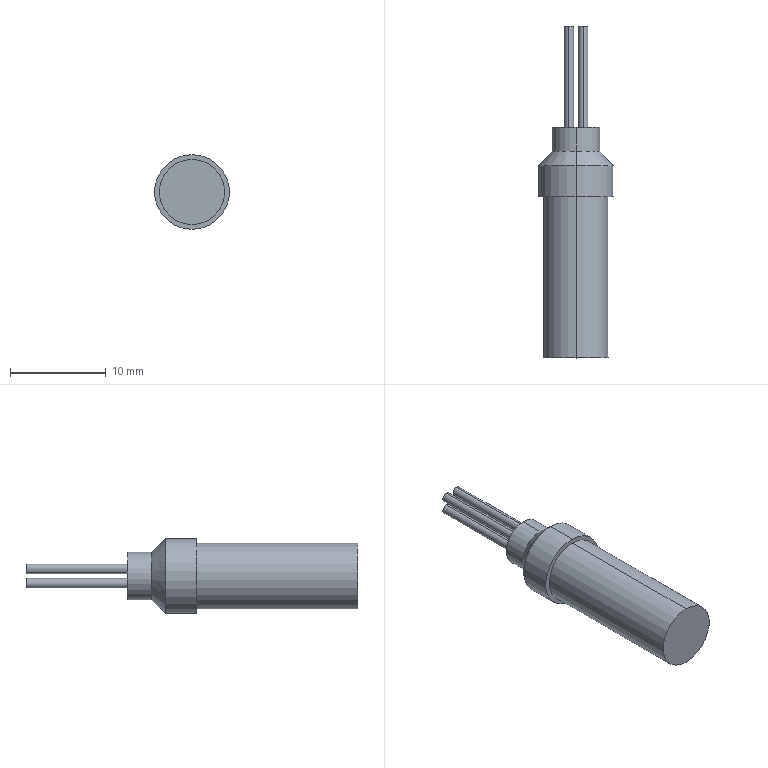Part | STEP file | Cable_Motor_Top_03_MSMF | 1 solid | 23 faces | box 7.8 x 34.633 x 7.8 mm | volume 896.959 mm3 | cylinder 14 | plane 7 | cone 2 | commonest cylinder face diameters 1 x8 5 x2 6.799 x2 7.8 x2
STEP:
#1=CARTESIAN_POINT('',(0.,0.,0.));
#2=DIRECTION('',(0.,0.,1.));
#3=DIRECTION('',(1.,0.,0.));
#4=AXIS2_PLACEMENT_3D('',#1,#2,#3);
#5=CARTESIAN_POINT('',(0.75,94.895,1.25));
#6=VERTEX_POINT('',#5);
#7=CARTESIAN_POINT('',(0.75,94.895,0.25));
#8=VERTEX_POINT('',#7);
#9=CARTESIAN_POINT('',(0.75,94.895,0.75));
#10=DIRECTION('',(0.,1.,0.));
#11=DIRECTION('',(0.,0.,1.));
#12=AXIS2_PLACEMENT_3D('',#9,#10,#11);
#13=CIRCLE('',#12,0.5);
#14=CARTESIAN_POINT('',(0.75,94.895,0.75));
#15=DIRECTION('',(0.,-1.,0.));
#16=DIRECTION('',(0.,0.,-1.));
#17=AXIS2_PLACEMENT_3D('',#14,#15,#16);
#18=CYLINDRICAL_SURFACE('',#17,0.5);
#19=CARTESIAN_POINT('',(3.142,0.));
#20=DIRECTION('',(-1.,0.));
#21=VECTOR('',#20,1.);
#22=LINE('',#19,#21);
#23=(GEOMETRIC_REPRESENTATION_CONTEXT(2)PARAMETRIC_REPRESENTATION_CONTEXT()REPRESENTATION_CONTEXT('',''));
#24=DEFINITIONAL_REPRESENTATION('',(#22),#23);
#25=PCURVE('',#18,#24);
#26=CARTESIAN_POINT('',(0.75,94.895,0.75));
#27=DIRECTION('',(0.,1.,0.));
#28=DIRECTION('',(0.,0.,1.));
#29=AXIS2_PLACEMENT_3D('',#26,#27,#28);
#30=PLANE('',#29);
#31=CARTESIAN_POINT('',(0.,0.));
#32=DIRECTION('',(1.,0.));
#33=AXIS2_PLACEMENT_2D('',#31,#32);
#34=CIRCLE('',#33,0.5);
#35=(GEOMETRIC_REPRESENTATION_CONTEXT(2)PARAMETRIC_REPRESENTATION_CONTEXT()REPRESENTATION_CONTEXT('',''));
#36=DEFINITIONAL_REPRESENTATION('',(#34),#35);
#37=PCURVE('',#30,#36);
#38=SURFACE_CURVE('',#13,(#25,#37),.PCURVE_S1.);
#39=EDGE_CURVE('',#6,#8,#38,.T.);
#40=ORIENTED_EDGE('',*,*,#39,.F.);
#41=CARTESIAN_POINT('',(0.75,84.322,1.25));
#42=VERTEX_POINT('',#41);
#43=CARTESIAN_POINT('',(0.75,94.895,1.25));
#44=DIRECTION('',(0.,-1.,0.));
#45=VECTOR('',#44,1.);
#46=LINE('',#43,#45);
#47=CARTESIAN_POINT('',(3.142,0.));
#48=DIRECTION('',(0.,1.));
#49=VECTOR('',#48,1.);
#50=LINE('',#47,#49);
#51=(GEOMETRIC_REPRESENTATION_CONTEXT(2)PARAMETRIC_REPRESENTATION_CONTEXT()REPRESENTATION_CONTEXT('',''));
#52=DEFINITIONAL_REPRESENTATION('',(#50),#51);
#53=PCURVE('',#18,#52);
#54=CARTESIAN_POINT('',(0.75,94.895,0.75));
#55=DIRECTION('',(0.,-1.,0.));
#56=DIRECTION('',(0.,0.,-1.));
#57=AXIS2_PLACEMENT_3D('',#54,#55,#56);
#58=CYLINDRICAL_SURFACE('',#57,0.5);
#59=CARTESIAN_POINT('',(3.142,0.));
#60=DIRECTION('',(0.,1.));
#61=VECTOR('',#60,1.);
#62=LINE('',#59,#61);
#63=(GEOMETRIC_REPRESENTATION_CONTEXT(2)PARAMETRIC_REPRESENTATION_CONTEXT()REPRESENTATION_CONTEXT('',''));
#64=DEFINITIONAL_REPRESENTATION('',(#62),#63);
#65=PCURVE('',#58,#64);
#66=SURFACE_CURVE('',#46,(#53,#65),.PCURVE_S1.);
#67=EDGE_CURVE('',#6,#42,#66,.T.);
#68=ORIENTED_EDGE('',*,*,#67,.T.);
#69=CARTESIAN_POINT('',(0.75,84.322,0.25));
#70=VERTEX_POINT('',#69);
#71=CARTESIAN_POINT('',(0.75,84.322,0.75));
#72=DIRECTION('',(0.,1.,0.));
#73=DIRECTION('',(0.,0.,-1.));
#74=AXIS2_PLACEMENT_3D('',#71,#72,#73);
#75=CIRCLE('',#74,0.5);
#76=CARTESIAN_POINT('',(6.283,10.573));
#77=DIRECTION('',(-1.,0.));
#78=VECTOR('',#77,1.);
#79=LINE('',#76,#78);
#80=(GEOMETRIC_REPRESENTATION_CONTEXT(2)PARAMETRIC_REPRESENTATION_CONTEXT()REPRESENTATION_CONTEXT('',''));
#81=DEFINITIONAL_REPRESENTATION('',(#79),#80);
#82=PCURVE('',#18,#81);
#83=CARTESIAN_POINT('',(0.,84.322,0.));
#84=DIRECTION('',(0.,-1.,0.));
#85=DIRECTION('',(0.,0.,-1.));
#86=AXIS2_PLACEMENT_3D('',#83,#84,#85);
#87=PLANE('',#86);
#88=CARTESIAN_POINT('',(-0.25,0.75));
#89=CARTESIAN_POINT('',(-0.25,-0.116));
#90=CARTESIAN_POINT('',(-1.,0.317));
#91=CARTESIAN_POINT('',(-1.75,0.75));
#92=CARTESIAN_POINT('',(-1.,1.183));
#93=CARTESIAN_POINT('',(-0.25,1.616));
#94=CARTESIAN_POINT('',(-0.25,0.75));
#95=(BOUNDED_CURVE()B_SPLINE_CURVE(2,(#88,#89,#90,#91,#92,#93,#94),.UNSPECIFIED.,.T.,.F.)B_SPLINE_CURVE_WITH_KNOTS((1,2,2,2,2,1),(-2.094,0.,2.094,4.189,6.283,8.378),.UNSPECIFIED.)CURVE()GEOMETRIC_REPRESENTATION_ITEM()RATIONAL_B_SPLINE_CURVE((1.,0.5,1.,0.5,1.,0.5,1.))REPRESENTATION_ITEM(''));
#96=(GEOMETRIC_REPRESENTATION_CONTEXT(2)PARAMETRIC_REPRESENTATION_CONTEXT()REPRESENTATION_CONTEXT('',''));
#97=DEFINITIONAL_REPRESENTATION('',(#95),#96);
#98=PCURVE('',#87,#97);
#99=SURFACE_CURVE('',#75,(#82,#98),.PCURVE_S1.);
#100=EDGE_CURVE('',#42,#70,#99,.T.);
#101=ORIENTED_EDGE('',*,*,#100,.T.);
#102=CARTESIAN_POINT('',(0.75,94.895,0.25));
#103=DIRECTION('',(0.,-1.,0.));
#104=VECTOR('',#103,1.);
#105=LINE('',#102,#104);
#106=CARTESIAN_POINT('',(0.,0.));
#107=DIRECTION('',(0.,1.));
#108=VECTOR('',#107,1.);
#109=LINE('',#106,#108);
#110=(GEOMETRIC_REPRESENTATION_CONTEXT(2)PARAMETRIC_REPRESENTATION_CONTEXT()REPRESENTATION_CONTEXT('',''));
#111=DEFINITIONAL_REPRESENTATION('',(#109),#110);
#112=PCURVE('',#18,#111);
#113=CARTESIAN_POINT('',(6.283,0.));
#114=DIRECTION('',(0.,1.));
#115=VECTOR('',#114,1.);
#116=LINE('',#113,#115);
#117=(GEOMETRIC_REPRESENTATION_CONTEXT(2)PARAMETRIC_REPRESENTATION_CONTEXT()REPRESENTATION_CONTEXT('',''));
#118=DEFINITIONAL_REPRESENTATION('',(#116),#117);
#119=PCURVE('',#58,#118);
#120=SURFACE_CURVE('',#105,(#112,#119),.PCURVE_S1.);
#121=EDGE_CURVE('',#8,#70,#120,.T.);
#122=ORIENTED_EDGE('',*,*,#121,.F.);
#123=EDGE_LOOP('',(#40,#68,#101,#122));
#124=FACE_BOUND('',#123,.T.);
#125=ADVANCED_FACE('',(#124),#18,.T.);
#126=CARTESIAN_POINT('',(-0.75,94.895,1.25));
#127=VERTEX_POINT('',#126);
#128=CARTESIAN_POINT('',(-0.75,94.895,0.25));
#129=VERTEX_POINT('',#128);
#130=CARTESIAN_POINT('',(-0.75,94.895,0.75));
#131=DIRECTION('',(0.,1.,0.));
#132=DIRECTION('',(0.,0.,1.));
#133=AXIS2_PLACEMENT_3D('',#130,#131,#132);
#134=CIRCLE('',#133,0.5);
#135=CARTESIAN_POINT('',(-0.75,94.895,0.75));
#136=DIRECTION('',(0.,-1.,0.));
#137=DIRECTION('',(0.,0.,-1.));
#138=AXIS2_PLACEMENT_3D('',#135,#136,#137);
#139=CYLINDRICAL_SURFACE('',#138,0.5);
#140=CARTESIAN_POINT('',(3.142,0.));
#141=DIRECTION('',(-1.,0.));
#142=VECTOR('',#141,1.);
#143=LINE('',#140,#142);
#144=(GEOMETRIC_REPRESENTATION_CONTEXT(2)PARAMETRIC_REPRESENTATION_CONTEXT()REPRESENTATION_CONTEXT('',''));
#145=DEFINITIONAL_REPRESENTATION('',(#143),#144);
#146=PCURVE('',#139,#145);
#147=CARTESIAN_POINT('',(-0.75,94.895,0.75));
#148=DIRECTION('',(0.,1.,0.));
#149=DIRECTION('',(0.,0.,1.));
#150=AXIS2_PLACEMENT_3D('',#147,#148,#149);
#151=PLANE('',#150);
#152=CARTESIAN_POINT('',(0.,0.));
#153=DIRECTION('',(1.,0.));
#154=AXIS2_PLACEMENT_2D('',#152,#153);
#155=CIRCLE('',#154,0.5);
#156=(GEOMETRIC_REPRESENTATION_CONTEXT(2)PARAMETRIC_REPRESENTATION_CONTEXT()REPRESENTATION_CONTEXT('',''));
#157=DEFINITIONAL_REPRESENTATION('',(#155),#156);
#158=PCURVE('',#151,#157);
#159=SURFACE_CURVE('',#134,(#146,#158),.PCURVE_S1.);
#160=EDGE_CURVE('',#127,#129,#159,.T.);
#161=ORIENTED_EDGE('',*,*,#160,.F.);
#162=CARTESIAN_POINT('',(-0.75,84.322,1.25));
#163=VERTEX_POINT('',#162);
#164=CARTESIAN_POINT('',(-0.75,94.895,1.25));
#165=DIRECTION('',(0.,-1.,0.));
#166=VECTOR('',#165,1.);
#167=LINE('',#164,#166);
#168=CARTESIAN_POINT('',(3.142,0.));
#169=DIRECTION('',(0.,1.));
#170=VECTOR('',#169,1.);
#171=LINE('',#168,#170);
#172=(GEOMETRIC_REPRESENTATION_CONTEXT(2)PARAMETRIC_REPRESENTATION_CONTEXT()REPRESENTATION_CONTEXT('',''));
#173=DEFINITIONAL_REPRESENTATION('',(#171),#172);
#174=PCURVE('',#139,#173);
#175=CARTESIAN_POINT('',(-0.75,94.895,0.75));
#176=DIRECTION('',(0.,-1.,0.));
#177=DIRECTION('',(0.,0.,-1.));
#178=AXIS2_PLACEMENT_3D('',#175,#176,#177);
#179=CYLINDRICAL_SURFACE('',#178,0.5);
#180=CARTESIAN_POINT('',(3.142,0.));
#181=DIRECTION('',(0.,1.));
#182=VECTOR('',#181,1.);
#183=LINE('',#180,#182);
#184=(GEOMETRIC_REPRESENTATION_CONTEXT(2)PARAMETRIC_REPRESENTATION_CONTEXT()REPRESENTATION_CONTEXT('',''));
#185=DEFINITIONAL_REPRESENTATION('',(#183),#184);
#186=PCURVE('',#179,#185);
#187=SURFACE_CURVE('',#167,(#174,#186),.PCURVE_S1.);
#188=EDGE_CURVE('',#127,#163,#187,.T.);
#189=ORIENTED_EDGE('',*,*,#188,.T.);
#190=CARTESIAN_POINT('',(-0.75,84.322,0.25));
#191=VERTEX_POINT('',#190);
#192=CARTESIAN_POINT('',(-0.75,84.322,0.75));
#193=DIRECTION('',(0.,1.,0.));
#194=DIRECTION('',(0.,0.,-1.));
#195=AXIS2_PLACEMENT_3D('',#192,#193,#194);
#196=CIRCLE('',#195,0.5);
#197=CARTESIAN_POINT('',(6.283,10.573));
#198=DIRECTION('',(-1.,0.));
#199=VECTOR('',#198,1.);
#200=LINE('',#197,#199);
#201=(GEOMETRIC_REPRESENTATION_CONTEXT(2)PARAMETRIC_REPRESENTATION_CONTEXT()REPRESENTATION_CONTEXT('',''));
#202=DEFINITIONAL_REPRESENTATION('',(#200),#201);
#203=PCURVE('',#139,#202);
#204=CARTESIAN_POINT('',(-0.25,-0.75));
#205=CARTESIAN_POINT('',(-0.25,-1.616));
#206=CARTESIAN_POINT('',(-1.,-1.183));
#207=CARTESIAN_POINT('',(-1.75,-0.75));
#208=CARTESIAN_POINT('',(-1.,-0.317));
#209=CARTESIAN_POINT('',(-0.25,0.116));
#210=CARTESIAN_POINT('',(-0.25,-0.75));
#211=(BOUNDED_CURVE()B_SPLINE_CURVE(2,(#204,#205,#206,#207,#208,#209,#210),.UNSPECIFIED.,.T.,.F.)B_SPLINE_CURVE_WITH_KNOTS((1,2,2,2,2,1),(-2.094,0.,2.094,4.189,6.283,8.378),.UNSPECIFIED.)CURVE()GEOMETRIC_REPRESENTATION_ITEM()RATIONAL_B_SPLINE_CURVE((1.,0.5,1.,0.5,1.,0.5,1.))REPRESENTATION_ITEM(''));
#212=(GEOMETRIC_REPRESENTATION_CONTEXT(2)PARAMETRIC_REPRESENTATION_CONTEXT()REPRESENTATION_CONTEXT('',''));
#213=DEFINITIONAL_REPRESENTATION('',(#211),#212);
#214=PCURVE('',#87,#213);
#215=SURFACE_CURVE('',#196,(#203,#214),.PCURVE_S1.);
#216=EDGE_CURVE('',#163,#191,#215,.T.);
#217=ORIENTED_EDGE('',*,*,#216,.T.);
#218=CARTESIAN_POINT('',(-0.75,94.895,0.25));
#219=DIRECTION('',(0.,-1.,0.));
#220=VECTOR('',#219,1.);
#221=LINE('',#218,#220);
#222=CARTESIAN_POINT('',(0.,0.));
#223=DIRECTION('',(0.,1.));
#224=VECTOR('',#223,1.);
#225=LINE('',#222,#224);
#226=(GEOMETRIC_REPRESENTATION_CONTEXT(2)PARAMETRIC_REPRESENTATION_CONTEXT()REPRESENTATION_CONTEXT('',''));
#227=DEFINITIONAL_REPRESENTATION('',(#225),#226);
#228=PCURVE('',#139,#227);
#229=CARTESIAN_POINT('',(6.283,0.));
#230=DIRECTION('',(0.,1.));
#231=VECTOR('',#230,1.);
#232=LINE('',#229,#231);
#233=(GEOMETRIC_REPRESENTATION_CONTEXT(2)PARAMETRIC_REPRESENTATION_CONTEXT()REPRESENTATION_CONTEXT('',''));
#234=DEFINITIONAL_REPRESENTATION('',(#232),#233);
#235=PCURVE('',#179,#234);
#236=SURFACE_CURVE('',#221,(#228,#235),.PCURVE_S1.);
#237=EDGE_CURVE('',#129,#191,#236,.T.);
#238=ORIENTED_EDGE('',*,*,#237,.F.);
#239=EDGE_LOOP('',(#161,#189,#217,#238));
#240=FACE_BOUND('',#239,.T.);
#241=ADVANCED_FACE('',(#240),#139,.T.);
#242=CARTESIAN_POINT('',(-0.75,94.895,-0.25));
#243=VERTEX_POINT('',#242);
#244=CARTESIAN_POINT('',(-0.75,94.895,-1.25));
#245=VERTEX_POINT('',#244);
#246=CARTESIAN_POINT('',(-0.75,94.895,-0.75));
#247=DIRECTION('',(0.,1.,0.));
#248=DIRECTION('',(0.,0.,1.));
#249=AXIS2_PLACEMENT_3D('',#246,#247,#248);
#250=CIRCLE('',#249,0.5);
#251=CARTESIAN_POINT('',(-0.75,94.895,-0.75));
#252=DIRECTION('',(0.,-1.,0.));
#253=DIRECTION('',(0.,0.,-1.));
#254=AXIS2_PLACEMENT_3D('',#251,#252,#253);
#255=CYLINDRICAL_SURFACE('',#254,0.5);
#256=CARTESIAN_POINT('',(3.142,0.));
#257=DIRECTION('',(-1.,0.));
#258=VECTOR('',#257,1.);
#259=LINE('',#256,#258);
#260=(GEOMETRIC_REPRESENTATION_CONTEXT(2)PARAMETRIC_REPRESENTATION_CONTEXT()REPRESENTATION_CONTEXT('',''));
#261=DEFINITIONAL_REPRESENTATION('',(#259),#260);
#262=PCURVE('',#255,#261);
#263=CARTESIAN_POINT('',(-0.75,94.895,-0.75));
#264=DIRECTION('',(0.,1.,0.));
#265=DIRECTION('',(0.,0.,1.));
#266=AXIS2_PLACEMENT_3D('',#263,#264,#265);
#267=PLANE('',#266);
#268=CARTESIAN_POINT('',(0.,0.));
#269=DIRECTION('',(1.,0.));
#270=AXIS2_PLACEMENT_2D('',#268,#269);
#271=CIRCLE('',#270,0.5);
#272=(GEOMETRIC_REPRESENTATION_CONTEXT(2)PARAMETRIC_REPRESENTATION_CONTEXT()REPRESENTATION_CONTEXT('',''));
#273=DEFINITIONAL_REPRESENTATION('',(#271),#272);
#274=PCURVE('',#267,#273);
#275=SURFACE_CURVE('',#250,(#262,#274),.PCURVE_S1.);
#276=EDGE_CURVE('',#243,#245,#275,.T.);
#277=ORIENTED_EDGE('',*,*,#276,.F.);
#278=CARTESIAN_POINT('',(-0.75,84.322,-0.25));
#279=VERTEX_POINT('',#278);
#280=CARTESIAN_POINT('',(-0.75,94.895,-0.25));
#281=DIRECTION('',(0.,-1.,0.));
#282=VECTOR('',#281,1.);
#283=LINE('',#280,#282);
#284=CARTESIAN_POINT('',(3.142,0.));
#285=DIRECTION('',(0.,1.));
#286=VECTOR('',#285,1.);
#287=LINE('',#284,#286);
#288=(GEOMETRIC_REPRESENTATION_CONTEXT(2)PARAMETRIC_REPRESENTATION_CONTEXT()REPRESENTATION_CONTEXT('',''));
#289=DEFINITIONAL_REPRESENTATION('',(#287),#288);
#290=PCURVE('',#255,#289);
#291=CARTESIAN_POINT('',(-0.75,94.895,-0.75));
#292=DIRECTION('',(0.,-1.,0.));
#293=DIRECTION('',(0.,0.,-1.));
#294=AXIS2_PLACEMENT_3D('',#291,#292,#293);
#295=CYLINDRICAL_SURFACE('',#294,0.5);
#296=CARTESIAN_POINT('',(3.142,0.));
#297=DIRECTION('',(0.,1.));
#298=VECTOR('',#297,1.);
#299=LINE('',#296,#298);
#300=(GEOMETRIC_REPRESENTATION_CONTEXT(2)PARAMETRIC_REPRESENTATION_CONTEXT()REPRESENTATION_CONTEXT('',''));
#301=DEFINITIONAL_REPRESENTATION('',(#299),#300);
#302=PCURVE('',#295,#301);
#303=SURFACE_CURVE('',#283,(#290,#302),.PCURVE_S1.);
#304=EDGE_CURVE('',#243,#279,#303,.T.);
#305=ORIENTED_EDGE('',*,*,#304,.T.);
#306=CARTESIAN_POINT('',(-0.75,84.322,-1.25));
#307=VERTEX_POINT('',#306);
#308=CARTESIAN_POINT('',(-0.75,84.322,-0.75));
#309=DIRECTION('',(0.,1.,0.));
#310=DIRECTION('',(0.,0.,-1.));
#311=AXIS2_PLACEMENT_3D('',#308,#309,#310);
#312=CIRCLE('',#311,0.5);
#313=CARTESIAN_POINT('',(6.283,10.573));
#314=DIRECTION('',(-1.,0.));
#315=VECTOR('',#314,1.);
#316=LINE('',#313,#315);
#317=(GEOMETRIC_REPRESENTATION_CONTEXT(2)PARAMETRIC_REPRESENTATION_CONTEXT()REPRESENTATION_CONTEXT('',''));
#318=DEFINITIONAL_REPRESENTATION('',(#316),#317);
#319=PCURVE('',#255,#318);
#320=CARTESIAN_POINT('',(1.25,-0.75));
#321=CARTESIAN_POINT('',(1.25,-1.616));
#322=CARTESIAN_POINT('',(0.5,-1.183));
#323=CARTESIAN_POINT('',(-0.25,-0.75));
#324=CARTESIAN_POINT('',(0.5,-0.317));
#325=CARTESIAN_POINT('',(1.25,0.116));
#326=CARTESIAN_POINT('',(1.25,-0.75));
#327=(BOUNDED_CURVE()B_SPLINE_CURVE(2,(#320,#321,#322,#323,#324,#325,#326),.UNSPECIFIED.,.T.,.F.)B_SPLINE_CURVE_WITH_KNOTS((1,2,2,2,2,1),(-2.094,0.,2.094,4.189,6.283,8.378),.UNSPECIFIED.)CURVE()GEOMETRIC_REPRESENTATION_ITEM()RATIONAL_B_SPLINE_CURVE((1.,0.5,1.,0.5,1.,0.5,1.))REPRESENTATION_ITEM(''));
#328=(GEOMETRIC_REPRESENTATION_CONTEXT(2)PARAMETRIC_REPRESENTATION_CONTEXT()REPRESENTATION_CONTEXT('',''));
#329=DEFINITIONAL_REPRESENTATION('',(#327),#328);
#330=PCURVE('',#87,#329);
#331=SURFACE_CURVE('',#312,(#319,#330),.PCURVE_S1.);
#332=EDGE_CURVE('',#279,#307,#331,.T.);
#333=ORIENTED_EDGE('',*,*,#332,.T.);
#334=CARTESIAN_POINT('',(-0.75,94.895,-1.25));
#335=DIRECTION('',(0.,-1.,0.));
#336=VECTOR('',#335,1.);
#337=LINE('',#334,#336);
#338=CARTESIAN_POINT('',(0.,0.));
#339=DIRECTION('',(0.,1.));
#340=VECTOR('',#339,1.);
#341=LINE('',#338,#340);
#342=(GEOMETRIC_REPRESENTATION_CONTEXT(2)PARAMETRIC_REPRESENTATION_CONTEXT()REPRESENTATION_CONTEXT('',''));
#343=DEFINITIONAL_REPRESENTATION('',(#341),#342);
#344=PCURVE('',#255,#343);
#345=CARTESIAN_POINT('',(6.283,0.));
#346=DIRECTION('',(0.,1.));
#347=VECTOR('',#346,1.);
#348=LINE('',#345,#347);
#349=(GEOMETRIC_REPRESENTATION_CONTEXT(2)PARAMETRIC_REPRESENTATION_CONTEXT()REPRESENTATION_CONTEXT('',''));
#350=DEFINITIONAL_REPRESENTATION('',(#348),#349);
#351=PCURVE('',#295,#350);
#352=SURFACE_CURVE('',#337,(#344,#351),.PCURVE_S1.);
#353=EDGE_CURVE('',#245,#307,#352,.T.);
#354=ORIENTED_EDGE('',*,*,#353,.F.);
#355=EDGE_LOOP('',(#277,#305,#333,#354));
#356=FACE_BOUND('',#355,.T.);
#357=ADVANCED_FACE('',(#356),#255,.T.);
#358=CARTESIAN_POINT('',(0.75,94.895,-0.25));
#359=VERTEX_POINT('',#358);
#360=CARTESIAN_POINT('',(0.75,94.895,-1.25));
#361=VERTEX_POINT('',#360);
#362=CARTESIAN_POINT('',(0.75,94.895,-0.75));
#363=DIRECTION('',(0.,1.,0.));
#364=DIRECTION('',(0.,0.,1.));
#365=AXIS2_PLACEMENT_3D('',#362,#363,#364);
#366=CIRCLE('',#365,0.5);
#367=CARTESIAN_POINT('',(0.75,94.895,-0.75));
#368=DIRECTION('',(0.,-1.,0.));
#369=DIRECTION('',(0.,0.,-1.));
#370=AXIS2_PLACEMENT_3D('',#367,#368,#369);
#371=CYLINDRICAL_SURFACE('',#370,0.5);
#372=CARTESIAN_POINT('',(3.142,0.));
#373=DIRECTION('',(-1.,0.));
#374=VECTOR('',#373,1.);
#375=LINE('',#372,#374);
#376=(GEOMETRIC_REPRESENTATION_CONTEXT(2)PARAMETRIC_REPRESENTATION_CONTEXT()REPRESENTATION_CONTEXT('',''));
#377=DEFINITIONAL_REPRESENTATION('',(#375),#376);
#378=PCURVE('',#371,#377);
#379=CARTESIAN_POINT('',(0.75,94.895,-0.75));
#380=DIRECTION('',(0.,1.,0.));
#381=DIRECTION('',(0.,0.,1.));
#382=AXIS2_PLACEMENT_3D('',#379,#380,#381);
#383=PLANE('',#382);
#384=CARTESIAN_POINT('',(0.,0.));
#385=DIRECTION('',(1.,0.));
#386=AXIS2_PLACEMENT_2D('',#384,#385);
#387=CIRCLE('',#386,0.5);
#388=(GEOMETRIC_REPRESENTATION_CONTEXT(2)PARAMETRIC_REPRESENTATION_CONTEXT()REPRESENTATION_CONTEXT('',''));
#389=DEFINITIONAL_REPRESENTATION('',(#387),#388);
#390=PCURVE('',#383,#389);
#391=SURFACE_CURVE('',#366,(#378,#390),.PCURVE_S1.);
#392=EDGE_CURVE('',#359,#361,#391,.T.);
#393=ORIENTED_EDGE('',*,*,#392,.F.);
#394=CARTESIAN_POINT('',(0.75,84.322,-0.25));
#395=VERTEX_POINT('',#394);
#396=CARTESIAN_POINT('',(0.75,94.895,-0.25));
#397=DIRECTION('',(0.,-1.,0.));
#398=VECTOR('',#397,1.);
#399=LINE('',#396,#398);
#400=CARTESIAN_POINT('',(3.142,0.));
#401=DIRECTION('',(0.,1.));
#402=VECTOR('',#401,1.);
#403=LINE('',#400,#402);
#404=(GEOMETRIC_REPRESENTATION_CONTEXT(2)PARAMETRIC_REPRESENTATION_CONTEXT()REPRESENTATION_CONTEXT('',''));
#405=DEFINITIONAL_REPRESENTATION('',(#403),#404);
#406=PCURVE('',#371,#405);
#407=CARTESIAN_POINT('',(0.75,94.895,-0.75));
#408=DIRECTION('',(0.,-1.,0.));
#409=DIRECTION('',(0.,0.,-1.));
#410=AXIS2_PLACEMENT_3D('',#407,#408,#409);
#411=CYLINDRICAL_SURFACE('',#410,0.5);
#412=CARTESIAN_POINT('',(3.142,0.));
#413=DIRECTION('',(0.,1.));
#414=VECTOR('',#413,1.);
#415=LINE('',#412,#414);
#416=(GEOMETRIC_REPRESENTATION_CONTEXT(2)PARAMETRIC_REPRESENTATION_CONTEXT()REPRESENTATION_CONTEXT('',''));
#417=DEFINITIONAL_REPRESENTATION('',(#415),#416);
#418=PCURVE('',#411,#417);
#419=SURFACE_CURVE('',#399,(#406,#418),.PCURVE_S1.);
#420=EDGE_CURVE('',#359,#395,#419,.T.);
#421=ORIENTED_EDGE('',*,*,#420,.T.);
#422=CARTESIAN_POINT('',(0.75,84.322,-1.25));
#423=VERTEX_POINT('',#422);
#424=CARTESIAN_POINT('',(0.75,84.322,-0.75));
#425=DIRECTION('',(0.,1.,0.));
#426=DIRECTION('',(0.,0.,-1.));
#427=AXIS2_PLACEMENT_3D('',#424,#425,#426);
#428=CIRCLE('',#427,0.5);
#429=CARTESIAN_POINT('',(6.283,10.573));
#430=DIRECTION('',(-1.,0.));
#431=VECTOR('',#430,1.);
#432=LINE('',#429,#431);
#433=(GEOMETRIC_REPRESENTATION_CONTEXT(2)PARAMETRIC_REPRESENTATION_CONTEXT()REPRESENTATION_CONTEXT('',''));
#434=DEFINITIONAL_REPRESENTATION('',(#432),#433);
#435=PCURVE('',#371,#434);
#436=CARTESIAN_POINT('',(1.25,0.75));
#437=CARTESIAN_POINT('',(1.25,-0.116));
#438=CARTESIAN_POINT('',(0.5,0.317));
#439=CARTESIAN_POINT('',(-0.25,0.75));
#440=CARTESIAN_POINT('',(0.5,1.183));
#441=CARTESIAN_POINT('',(1.25,1.616));
#442=CARTESIAN_POINT('',(1.25,0.75));
#443=(BOUNDED_CURVE()B_SPLINE_CURVE(2,(#436,#437,#438,#439,#440,#441,#442),.UNSPECIFIED.,.T.,.F.)B_SPLINE_CURVE_WITH_KNOTS((1,2,2,2,2,1),(-2.094,0.,2.094,4.189,6.283,8.378),.UNSPECIFIED.)CURVE()GEOMETRIC_REPRESENTATION_ITEM()RATIONAL_B_SPLINE_CURVE((1.,0.5,1.,0.5,1.,0.5,1.))REPRESENTATION_ITEM(''));
#444=(GEOMETRIC_REPRESENTATION_CONTEXT(2)PARAMETRIC_REPRESENTATION_CONTEXT()REPRESENTATION_CONTEXT('',''));
#445=DEFINITIONAL_REPRESENTATION('',(#443),#444);
#446=PCURVE('',#87,#445);
#447=SURFACE_CURVE('',#428,(#435,#446),.PCURVE_S1.);
#448=EDGE_CURVE('',#395,#423,#447,.T.);
#449=ORIENTED_EDGE('',*,*,#448,.T.);
#450=CARTESIAN_POINT('',(0.75,94.895,-1.25));
#451=DIRECTION('',(0.,-1.,0.));
#452=VECTOR('',#451,1.);
#453=LINE('',#450,#452);
#454=CARTESIAN_POINT('',(0.,0.));
#455=DIRECTION('',(0.,1.));
#456=VECTOR('',#455,1.);
#457=LINE('',#454,#456);
#458=(GEOMETRIC_REPRESENTATION_CONTEXT(2)PARAMETRIC_REPRESENTATION_CONTEXT()REPRESENTATION_CONTEXT('',''));
#459=DEFINITIONAL_REPRESENTATION('',(#457),#458);
#460=PCURVE('',#371,#459);
#461=CARTESIAN_POINT('',(6.283,0.));
#462=DIRECTION('',(0.,1.));
#463=VECTOR('',#462,1.);
#464=LINE('',#461,#463);
#465=(GEOMETRIC_REPRESENTATION_CONTEXT(2)PARAMETRIC_REPRESENTATION_CONTEXT()REPRESENTATION_CONTEXT('',''));
#466=DEFINITIONAL_REPRESENTATION('',(#464),#465);
#467=PCURVE('',#411,#466);
#468=SURFACE_CURVE('',#453,(#460,#467),.PCURVE_S1.);
#469=EDGE_CURVE('',#361,#423,#468,.T.);
#470=ORIENTED_EDGE('',*,*,#469,.F.);
#471=EDGE_LOOP('',(#393,#421,#449,#470));
#472=FACE_BOUND('',#471,.T.);
#473=ADVANCED_FACE('',(#472),#371,.T.);
#474=CARTESIAN_POINT('',(0.,77.072,3.9));
#475=VERTEX_POINT('',#474);
#476=CARTESIAN_POINT('',(0.,77.072,-3.9));
#477=VERTEX_POINT('',#476);
#478=CARTESIAN_POINT('',(0.,77.072,0.));
#479=DIRECTION('',(0.,1.,0.));
#480=DIRECTION('',(0.,0.,1.));
#481=AXIS2_PLACEMENT_3D('',#478,#479,#480);
#482=CIRCLE('',#481,3.9);
#483=CARTESIAN_POINT('',(0.,77.072,0.));
#484=DIRECTION('',(0.,1.,0.));
#485=DIRECTION('',(0.,0.,1.));
#486=AXIS2_PLACEMENT_3D('',#483,#484,#485);
#487=CYLINDRICAL_SURFACE('',#486,3.9);
#488=CARTESIAN_POINT('',(0.,0.));
#489=DIRECTION('',(1.,0.));
#490=VECTOR('',#489,1.);
#491=LINE('',#488,#490);
#492=(GEOMETRIC_REPRESENTATION_CONTEXT(2)PARAMETRIC_REPRESENTATION_CONTEXT()REPRESENTATION_CONTEXT('',''));
#493=DEFINITIONAL_REPRESENTATION('',(#491),#492);
#494=PCURVE('',#487,#493);
#495=CARTESIAN_POINT('',(3.9,77.072,0.));
#496=DIRECTION('',(0.,1.,0.));
#497=DIRECTION('',(0.,0.,1.));
#498=AXIS2_PLACEMENT_3D('',#495,#496,#497);
#499=PLANE('',#498);
#500=CARTESIAN_POINT('',(0.,-3.9));
#501=DIRECTION('',(1.,0.));
#502=AXIS2_PLACEMENT_2D('',#500,#501);
#503=CIRCLE('',#502,3.9);
#504=(GEOMETRIC_REPRESENTATION_CONTEXT(2)PARAMETRIC_REPRESENTATION_CONTEXT()REPRESENTATION_CONTEXT('',''));
#505=DEFINITIONAL_REPRESENTATION('',(#503),#504);
#506=PCURVE('',#499,#505);
#507=SURFACE_CURVE('',#482,(#494,#506),.PCURVE_S1.);
#508=EDGE_CURVE('',#475,#477,#507,.T.);
#509=ORIENTED_EDGE('',*,*,#508,.T.);
#510=CARTESIAN_POINT('',(0.,80.322,-3.9));
#511=VERTEX_POINT('',#510);
#512=CARTESIAN_POINT('',(0.,77.072,-3.9));
#513=DIRECTION('',(0.,1.,0.));
#514=VECTOR('',#513,1.);
#515=LINE('',#512,#514);
#516=CARTESIAN_POINT('',(3.142,0.));
#517=DIRECTION('',(0.,1.));
#518=VECTOR('',#517,1.);
#519=LINE('',#516,#518);
#520=(GEOMETRIC_REPRESENTATION_CONTEXT(2)PARAMETRIC_REPRESENTATION_CONTEXT()REPRESENTATION_CONTEXT('',''));
#521=DEFINITIONAL_REPRESENTATION('',(#519),#520);
#522=PCURVE('',#487,#521);
#523=CARTESIAN_POINT('',(0.,77.072,0.));
#524=DIRECTION('',(0.,1.,0.));
#525=DIRECTION('',(0.,0.,1.));
#526=AXIS2_PLACEMENT_3D('',#523,#524,#525);
#527=CYLINDRICAL_SURFACE('',#526,3.9);
#528=CARTESIAN_POINT('',(3.142,0.));
#529=DIRECTION('',(0.,1.));
#530=VECTOR('',#529,1.);
#531=LINE('',#528,#530);
#532=(GEOMETRIC_REPRESENTATION_CONTEXT(2)PARAMETRIC_REPRESENTATION_CONTEXT()REPRESENTATION_CONTEXT('',''));
#533=DEFINITIONAL_REPRESENTATION('',(#531),#532);
#534=PCURVE('',#527,#533);
#535=SURFACE_CURVE('',#515,(#522,#534),.PCURVE_S1.);
#536=EDGE_CURVE('',#477,#511,#535,.T.);
#537=ORIENTED_EDGE('',*,*,#536,.T.);
#538=CARTESIAN_POINT('',(0.,80.322,3.9));
#539=VERTEX_POINT('',#538);
#540=CARTESIAN_POINT('',(0.,80.322,0.));
#541=DIRECTION('',(0.,1.,0.));
#542=DIRECTION('',(0.,0.,1.));
#543=AXIS2_PLACEMENT_3D('',#540,#541,#542);
#544=CIRCLE('',#543,3.9);
#545=CARTESIAN_POINT('',(0.,3.25));
#546=DIRECTION('',(1.,0.));
#547=VECTOR('',#546,1.);
#548=LINE('',#545,#547);
#549=(GEOMETRIC_REPRESENTATION_CONTEXT(2)PARAMETRIC_REPRESENTATION_CONTEXT()REPRESENTATION_CONTEXT('',''));
#550=DEFINITIONAL_REPRESENTATION('',(#548),#549);
#551=PCURVE('',#487,#550);
#552=CARTESIAN_POINT('',(0.,80.322,0.));
#553=DIRECTION('',(0.,-1.,0.));
#554=DIRECTION('',(0.,0.,-1.));
#555=AXIS2_PLACEMENT_3D('',#552,#553,#554);
#556=CONICAL_SURFACE('',#555,3.9,0.7509);
#557=CARTESIAN_POINT('',(3.142,0.));
#558=DIRECTION('',(-1.,0.));
#559=VECTOR('',#558,1.);
#560=LINE('',#557,#559);
#561=(GEOMETRIC_REPRESENTATION_CONTEXT(2)PARAMETRIC_REPRESENTATION_CONTEXT()REPRESENTATION_CONTEXT('',''));
#562=DEFINITIONAL_REPRESENTATION('',(#560),#561);
#563=PCURVE('',#556,#562);
#564=SURFACE_CURVE('',#544,(#551,#563),.PCURVE_S1.);
#565=EDGE_CURVE('',#539,#511,#564,.T.);
#566=ORIENTED_EDGE('',*,*,#565,.F.);
#567=CARTESIAN_POINT('',(0.,77.072,3.9));
#568=DIRECTION('',(0.,1.,0.));
#569=VECTOR('',#568,1.);
#570=LINE('',#567,#569);
#571=CARTESIAN_POINT('',(0.,0.));
#572=DIRECTION('',(0.,1.));
#573=VECTOR('',#572,1.);
#574=LINE('',#571,#573);
#575=(GEOMETRIC_REPRESENTATION_CONTEXT(2)PARAMETRIC_REPRESENTATION_CONTEXT()REPRESENTATION_CONTEXT('',''));
#576=DEFINITIONAL_REPRESENTATION('',(#574),#575);
#577=PCURVE('',#487,#576);
#578=CARTESIAN_POINT('',(6.283,0.));
#579=DIRECTION('',(0.,1.));
#580=VECTOR('',#579,1.);
#581=LINE('',#578,#580);
#582=(GEOMETRIC_REPRESENTATION_CONTEXT(2)PARAMETRIC_REPRESENTATION_CONTEXT()REPRESENTATION_CONTEXT('',''));
#583=DEFINITIONAL_REPRESENTATION('',(#581),#582);
#584=PCURVE('',#527,#583);
#585=SURFACE_CURVE('',#570,(#577,#584),.PCURVE_S1.);
#586=EDGE_CURVE('',#475,#539,#585,.T.);
#587=ORIENTED_EDGE('',*,*,#586,.F.);
#588=EDGE_LOOP('',(#509,#537,#566,#587));
#589=FACE_BOUND('',#588,.T.);
#590=ADVANCED_FACE('',(#589),#487,.T.);
#591=CARTESIAN_POINT('',(0.,81.822,2.5));
#592=VERTEX_POINT('',#591);
#593=CARTESIAN_POINT('',(0.,81.822,-2.5));
#594=VERTEX_POINT('',#593);
#595=CARTESIAN_POINT('',(0.,81.822,0.));
#596=DIRECTION('',(0.,1.,0.));
#597=DIRECTION('',(0.,0.,1.));
#598=AXIS2_PLACEMENT_3D('',#595,#596,#597);
#599=CIRCLE('',#598,2.5);
#600=CARTESIAN_POINT('',(3.142,-1.5));
#601=DIRECTION('',(-1.,0.));
#602=VECTOR('',#601,1.);
#603=LINE('',#600,#602);
#604=(GEOMETRIC_REPRESENTATION_CONTEXT(2)PARAMETRIC_REPRESENTATION_CONTEXT()REPRESENTATION_CONTEXT('',''));
#605=DEFINITIONAL_REPRESENTATION('',(#603),#604);
#606=PCURVE('',#556,#605);
#607=CARTESIAN_POINT('',(0.,77.072,0.));
#608=DIRECTION('',(0.,1.,0.));
#609=DIRECTION('',(0.,0.,1.));
#610=AXIS2_PLACEMENT_3D('',#607,#608,#609);
#611=CYLINDRICAL_SURFACE('',#610,2.5);
#612=CARTESIAN_POINT('',(0.,4.75));
#613=DIRECTION('',(1.,0.));
#614=VECTOR('',#613,1.);
#615=LINE('',#612,#614);
#616=(GEOMETRIC_REPRESENTATION_CONTEXT(2)PARAMETRIC_REPRESENTATION_CONTEXT()REPRESENTATION_CONTEXT('',''));
#617=DEFINITIONAL_REPRESENTATION('',(#615),#616);
#618=PCURVE('',#611,#617);
#619=SURFACE_CURVE('',#599,(#606,#618),.PCURVE_S1.);
#620=EDGE_CURVE('',#592,#594,#619,.T.);
#621=ORIENTED_EDGE('',*,*,#620,.F.);
#622=CARTESIAN_POINT('',(0.,80.322,3.9));
#623=DIRECTION('',(0.,-0.7311,0.6823));
#624=VECTOR('',#623,1.);
#625=LINE('',#622,#624);
#626=CARTESIAN_POINT('',(3.142,0.));
#627=DIRECTION('',(0.,1.));
#628=VECTOR('',#627,1.);
#629=LINE('',#626,#628);
#630=(GEOMETRIC_REPRESENTATION_CONTEXT(2)PARAMETRIC_REPRESENTATION_CONTEXT()REPRESENTATION_CONTEXT('',''));
#631=DEFINITIONAL_REPRESENTATION('',(#629),#630);
#632=PCURVE('',#556,#631);
#633=CARTESIAN_POINT('',(0.,80.322,0.));
#634=DIRECTION('',(0.,-1.,0.));
#635=DIRECTION('',(0.,0.,-1.));
#636=AXIS2_PLACEMENT_3D('',#633,#634,#635);
#637=CONICAL_SURFACE('',#636,3.9,0.7509);
#638=CARTESIAN_POINT('',(3.142,0.));
#639=DIRECTION('',(0.,1.));
#640=VECTOR('',#639,1.);
#641=LINE('',#638,#640);
#642=(GEOMETRIC_REPRESENTATION_CONTEXT(2)PARAMETRIC_REPRESENTATION_CONTEXT()REPRESENTATION_CONTEXT('',''));
#643=DEFINITIONAL_REPRESENTATION('',(#641),#642);
#644=PCURVE('',#637,#643);
#645=SURFACE_CURVE('',#625,(#632,#644),.PCURVE_S1.);
#646=EDGE_CURVE('',#592,#539,#645,.T.);
#647=ORIENTED_EDGE('',*,*,#646,.T.);
#648=ORIENTED_EDGE('',*,*,#565,.T.);
#649=CARTESIAN_POINT('',(0.,80.322,-3.9));
#650=DIRECTION('',(0.,-0.7311,-0.6823));
#651=VECTOR('',#650,1.);
#652=LINE('',#649,#651);
#653=CARTESIAN_POINT('',(0.,0.));
#654=DIRECTION('',(0.,1.));
#655=VECTOR('',#654,1.);
#656=LINE('',#653,#655);
#657=(GEOMETRIC_REPRESENTATION_CONTEXT(2)PARAMETRIC_REPRESENTATION_CONTEXT()REPRESENTATION_CONTEXT('',''));
#658=DEFINITIONAL_REPRESENTATION('',(#656),#657);
#659=PCURVE('',#556,#658);
#660=CARTESIAN_POINT('',(6.283,0.));
#661=DIRECTION('',(0.,1.));
#662=VECTOR('',#661,1.);
#663=LINE('',#660,#662);
#664=(GEOMETRIC_REPRESENTATION_CONTEXT(2)PARAMETRIC_REPRESENTATION_CONTEXT()REPRESENTATION_CONTEXT('',''));
#665=DEFINITIONAL_REPRESENTATION('',(#663),#664);
#666=PCURVE('',#637,#665);
#667=SURFACE_CURVE('',#652,(#659,#666),.PCURVE_S1.);
#668=EDGE_CURVE('',#594,#511,#667,.T.);
#669=ORIENTED_EDGE('',*,*,#668,.F.);
#670=EDGE_LOOP('',(#621,#647,#648,#669));
#671=FACE_BOUND('',#670,.T.);
#672=ADVANCED_FACE('',(#671),#556,.T.);
#673=ORIENTED_EDGE('',*,*,#620,.T.);
#674=CARTESIAN_POINT('',(0.,84.322,-2.5));
#675=VERTEX_POINT('',#674);
#676=CARTESIAN_POINT('',(0.,77.072,-2.5));
#677=DIRECTION('',(0.,1.,0.));
#678=VECTOR('',#677,1.);
#679=LINE('',#676,#678);
#680=CARTESIAN_POINT('',(3.142,0.));
#681=DIRECTION('',(0.,1.));
#682=VECTOR('',#681,1.);
#683=LINE('',#680,#682);
#684=(GEOMETRIC_REPRESENTATION_CONTEXT(2)PARAMETRIC_REPRESENTATION_CONTEXT()REPRESENTATION_CONTEXT('',''));
#685=DEFINITIONAL_REPRESENTATION('',(#683),#684);
#686=PCURVE('',#611,#685);
#687=CARTESIAN_POINT('',(0.,77.072,0.));
#688=DIRECTION('',(0.,1.,0.));
#689=DIRECTION('',(0.,0.,1.));
#690=AXIS2_PLACEMENT_3D('',#687,#688,#689);
#691=CYLINDRICAL_SURFACE('',#690,2.5);
#692=CARTESIAN_POINT('',(3.142,0.));
#693=DIRECTION('',(0.,1.));
#694=VECTOR('',#693,1.);
#695=LINE('',#692,#694);
#696=(GEOMETRIC_REPRESENTATION_CONTEXT(2)PARAMETRIC_REPRESENTATION_CONTEXT()REPRESENTATION_CONTEXT('',''));
#697=DEFINITIONAL_REPRESENTATION('',(#695),#696);
#698=PCURVE('',#691,#697);
#699=SURFACE_CURVE('',#679,(#686,#698),.PCURVE_S1.);
#700=EDGE_CURVE('',#594,#675,#699,.T.);
#701=ORIENTED_EDGE('',*,*,#700,.T.);
#702=CARTESIAN_POINT('',(0.,84.322,2.5));
#703=VERTEX_POINT('',#702);
#704=CARTESIAN_POINT('',(0.,84.322,0.));
#705=DIRECTION('',(0.,1.,0.));
#706=DIRECTION('',(0.,0.,1.));
#707=AXIS2_PLACEMENT_3D('',#704,#705,#706);
#708=CIRCLE('',#707,2.5);
#709=CARTESIAN_POINT('',(0.,7.25));
#710=DIRECTION('',(1.,0.));
#711=VECTOR('',#710,1.);
#712=LINE('',#709,#711);
#713=(GEOMETRIC_REPRESENTATION_CONTEXT(2)PARAMETRIC_REPRESENTATION_CONTEXT()REPRESENTATION_CONTEXT('',''));
#714=DEFINITIONAL_REPRESENTATION('',(#712),#713);
#715=PCURVE('',#611,#714);
#716=CARTESIAN_POINT('',(-2.5,0.));
#717=CARTESIAN_POINT('',(-2.5,4.33));
#718=CARTESIAN_POINT('',(1.25,2.165));
#719=CARTESIAN_POINT('',(5.,0.));
#720=CARTESIAN_POINT('',(1.25,-2.165));
#721=CARTESIAN_POINT('',(-2.5,-4.33));
#722=CARTESIAN_POINT('',(-2.5,0.));
#723=(BOUNDED_CURVE()B_SPLINE_CURVE(2,(#716,#717,#718,#719,#720,#721,#722),.UNSPECIFIED.,.T.,.F.)B_SPLINE_CURVE_WITH_KNOTS((1,2,2,2,2,1),(-2.094,0.,2.094,4.189,6.283,8.378),.UNSPECIFIED.)CURVE()GEOMETRIC_REPRESENTATION_ITEM()RATIONAL_B_SPLINE_CURVE((1.,0.5,1.,0.5,1.,0.5,1.))REPRESENTATION_ITEM(''));
#724=(GEOMETRIC_REPRESENTATION_CONTEXT(2)PARAMETRIC_REPRESENTATION_CONTEXT()REPRESENTATION_CONTEXT('',''));
#725=DEFINITIONAL_REPRESENTATION('',(#723),#724);
#726=PCURVE('',#87,#725);
#727=SURFACE_CURVE('',#708,(#715,#726),.PCURVE_S1.);
#728=EDGE_CURVE('',#703,#675,#727,.T.);
#729=ORIENTED_EDGE('',*,*,#728,.F.);
#730=CARTESIAN_POINT('',(0.,77.072,2.5));
#731=DIRECTION('',(0.,1.,0.));
#732=VECTOR('',#731,1.);
#733=LINE('',#730,#732);
#734=CARTESIAN_POINT('',(0.,0.));
#735=DIRECTION('',(0.,1.));
#736=VECTOR('',#735,1.);
#737=LINE('',#734,#736);
#738=(GEOMETRIC_REPRESENTATION_CONTEXT(2)PARAMETRIC_REPRESENTATION_CONTEXT()REPRESENTATION_CONTEXT('',''));
#739=DEFINITIONAL_REPRESENTATION('',(#737),#738);
#740=PCURVE('',#611,#739);
#741=CARTESIAN_POINT('',(6.283,0.));
#742=DIRECTION('',(0.,1.));
#743=VECTOR('',#742,1.);
#744=LINE('',#741,#743);
#745=(GEOMETRIC_REPRESENTATION_CONTEXT(2)PARAMETRIC_REPRESENTATION_CONTEXT()REPRESENTATION_CONTEXT('',''));
#746=DEFINITIONAL_REPRESENTATION('',(#744),#745);
#747=PCURVE('',#691,#746);
#748=SURFACE_CURVE('',#733,(#740,#747),.PCURVE_S1.);
#749=EDGE_CURVE('',#592,#703,#748,.T.);
#750=ORIENTED_EDGE('',*,*,#749,.F.);
#751=EDGE_LOOP('',(#673,#701,#729,#750));
#752=FACE_BOUND('',#751,.T.);
#753=ADVANCED_FACE('',(#752),#611,.T.);
#754=CARTESIAN_POINT('',(0.,77.072,3.4));
#755=VERTEX_POINT('',#754);
#756=CARTESIAN_POINT('',(0.,77.072,-3.4));
#757=VERTEX_POINT('',#756);
#758=CARTESIAN_POINT('',(0.,77.072,0.));
#759=DIRECTION('',(0.,1.,0.));
#760=DIRECTION('',(0.,0.,1.));
#761=AXIS2_PLACEMENT_3D('',#758,#759,#760);
#762=CIRCLE('',#761,3.4);
#763=CARTESIAN_POINT('',(0.,79.322,0.));
#764=DIRECTION('',(0.,-1.,0.));
#765=DIRECTION('',(0.,0.,-1.));
#766=AXIS2_PLACEMENT_3D('',#763,#764,#765);
#767=CYLINDRICAL_SURFACE('',#766,3.4);
#768=CARTESIAN_POINT('',(3.142,2.25));
#769=DIRECTION('',(-1.,0.));
#770=VECTOR('',#769,1.);
#771=LINE('',#768,#770);
#772=(GEOMETRIC_REPRESENTATION_CONTEXT(2)PARAMETRIC_REPRESENTATION_CONTEXT()REPRESENTATION_CONTEXT('',''));
#773=DEFINITIONAL_REPRESENTATION('',(#771),#772);
#774=PCURVE('',#767,#773);
#775=CARTESIAN_POINT('',(0.,-3.9));
#776=DIRECTION('',(1.,0.));
#777=AXIS2_PLACEMENT_2D('',#775,#776);
#778=CIRCLE('',#777,3.4);
#779=(GEOMETRIC_REPRESENTATION_CONTEXT(2)PARAMETRIC_REPRESENTATION_CONTEXT()REPRESENTATION_CONTEXT('',''));
#780=DEFINITIONAL_REPRESENTATION('',(#778),#779);
#781=PCURVE('',#499,#780);
#782=SURFACE_CURVE('',#762,(#774,#781),.PCURVE_S1.);
#783=EDGE_CURVE('',#755,#757,#782,.T.);
#784=ORIENTED_EDGE('',*,*,#783,.F.);
#785=CARTESIAN_POINT('',(0.,60.262,3.4));
#786=VERTEX_POINT('',#785);
#787=CARTESIAN_POINT('',(0.,79.322,3.4));
#788=DIRECTION('',(0.,-1.,0.));
#789=VECTOR('',#788,1.);
#790=LINE('',#787,#789);
#791=CARTESIAN_POINT('',(3.142,0.));
#792=DIRECTION('',(0.,1.));
#793=VECTOR('',#792,1.);
#794=LINE('',#791,#793);
#795=(GEOMETRIC_REPRESENTATION_CONTEXT(2)PARAMETRIC_REPRESENTATION_CONTEXT()REPRESENTATION_CONTEXT('',''));
#796=DEFINITIONAL_REPRESENTATION('',(#794),#795);
#797=PCURVE('',#767,#796);
#798=CARTESIAN_POINT('',(0.,79.322,0.));
#799=DIRECTION('',(0.,-1.,0.));
#800=DIRECTION('',(0.,0.,-1.));
#801=AXIS2_PLACEMENT_3D('',#798,#799,#800);
#802=CYLINDRICAL_SURFACE('',#801,3.4);
#803=CARTESIAN_POINT('',(3.142,0.));
#804=DIRECTION('',(0.,1.));
#805=VECTOR('',#804,1.);
#806=LINE('',#803,#805);
#807=(GEOMETRIC_REPRESENTATION_CONTEXT(2)PARAMETRIC_REPRESENTATION_CONTEXT()REPRESENTATION_CONTEXT('',''));
#808=DEFINITIONAL_REPRESENTATION('',(#806),#807);
#809=PCURVE('',#802,#808);
#810=SURFACE_CURVE('',#790,(#797,#809),.PCURVE_S1.);
#811=EDGE_CURVE('',#755,#786,#810,.T.);
#812=ORIENTED_EDGE('',*,*,#811,.T.);
#813=CARTESIAN_POINT('',(0.,60.262,-3.4));
#814=VERTEX_POINT('',#813);
#815=CARTESIAN_POINT('',(0.,60.262,0.));
#816=DIRECTION('',(0.,1.,0.));
#817=DIRECTION('',(0.,0.,1.));
#818=AXIS2_PLACEMENT_3D('',#815,#816,#817);
#819=CIRCLE('',#818,3.4);
#820=CARTESIAN_POINT('',(3.142,19.06));
#821=DIRECTION('',(-1.,0.));
#822=VECTOR('',#821,1.);
#823=LINE('',#820,#822);
#824=(GEOMETRIC_REPRESENTATION_CONTEXT(2)PARAMETRIC_REPRESENTATION_CONTEXT()REPRESENTATION_CONTEXT('',''));
#825=DEFINITIONAL_REPRESENTATION('',(#823),#824);
#826=PCURVE('',#767,#825);
#827=CARTESIAN_POINT('',(0.,60.262,0.));
#828=DIRECTION('',(0.,1.,0.));
#829=DIRECTION('',(0.,0.,1.));
#830=AXIS2_PLACEMENT_3D('',#827,#828,#829);
#831=PLANE('',#830);
#832=CARTESIAN_POINT('',(0.,0.));
#833=DIRECTION('',(1.,0.));
#834=AXIS2_PLACEMENT_2D('',#832,#833);
#835=CIRCLE('',#834,3.4);
#836=(GEOMETRIC_REPRESENTATION_CONTEXT(2)PARAMETRIC_REPRESENTATION_CONTEXT()REPRESENTATION_CONTEXT('',''));
#837=DEFINITIONAL_REPRESENTATION('',(#835),#836);
#838=PCURVE('',#831,#837);
#839=SURFACE_CURVE('',#819,(#826,#838),.PCURVE_S1.);
#840=EDGE_CURVE('',#786,#814,#839,.T.);
#841=ORIENTED_EDGE('',*,*,#840,.T.);
#842=CARTESIAN_POINT('',(0.,79.322,-3.4));
#843=DIRECTION('',(0.,-1.,0.));
#844=VECTOR('',#843,1.);
#845=LINE('',#842,#844);
#846=CARTESIAN_POINT('',(0.,0.));
#847=DIRECTION('',(0.,1.));
#848=VECTOR('',#847,1.);
#849=LINE('',#846,#848);
#850=(GEOMETRIC_REPRESENTATION_CONTEXT(2)PARAMETRIC_REPRESENTATION_CONTEXT()REPRESENTATION_CONTEXT('',''));
#851=DEFINITIONAL_REPRESENTATION('',(#849),#850);
#852=PCURVE('',#767,#851);
#853=CARTESIAN_POINT('',(6.283,0.));
#854=DIRECTION('',(0.,1.));
#855=VECTOR('',#854,1.);
#856=LINE('',#853,#855);
#857=(GEOMETRIC_REPRESENTATION_CONTEXT(2)PARAMETRIC_REPRESENTATION_CONTEXT()REPRESENTATION_CONTEXT('',''));
#858=DEFINITIONAL_REPRESENTATION('',(#856),#857);
#859=PCURVE('',#802,#858);
#860=SURFACE_CURVE('',#845,(#852,#859),.PCURVE_S1.);
#861=EDGE_CURVE('',#757,#814,#860,.T.);
#862=ORIENTED_EDGE('',*,*,#861,.F.);
#863=EDGE_LOOP('',(#784,#812,#841,#862));
#864=FACE_BOUND('',#863,.T.);
#865=ADVANCED_FACE('',(#864),#767,.T.);
#866=ORIENTED_EDGE('',*,*,#811,.F.);
#867=CARTESIAN_POINT('',(0.,77.072,0.));
#868=DIRECTION('',(0.,1.,0.));
#869=DIRECTION('',(0.,0.,1.));
#870=AXIS2_PLACEMENT_3D('',#867,#868,#869);
#871=CIRCLE('',#870,3.4);
#872=CARTESIAN_POINT('',(9.425,2.25));
#873=DIRECTION('',(-1.,0.));
#874=VECTOR('',#873,1.);
#875=LINE('',#872,#874);
#876=(GEOMETRIC_REPRESENTATION_CONTEXT(2)PARAMETRIC_REPRESENTATION_CONTEXT()REPRESENTATION_CONTEXT('',''));
#877=DEFINITIONAL_REPRESENTATION('',(#875),#876);
#878=PCURVE('',#802,#877);
#879=CARTESIAN_POINT('',(0.,-3.9));
#880=DIRECTION('',(1.,0.));
#881=AXIS2_PLACEMENT_2D('',#879,#880);
#882=CIRCLE('',#881,3.4);
#883=(GEOMETRIC_REPRESENTATION_CONTEXT(2)PARAMETRIC_REPRESENTATION_CONTEXT()REPRESENTATION_CONTEXT('',''));
#884=DEFINITIONAL_REPRESENTATION('',(#882),#883);
#885=PCURVE('',#499,#884);
#886=SURFACE_CURVE('',#871,(#878,#885),.PCURVE_S1.);
#887=EDGE_CURVE('',#757,#755,#886,.T.);
#888=ORIENTED_EDGE('',*,*,#887,.F.);
#889=ORIENTED_EDGE('',*,*,#861,.T.);
#890=CARTESIAN_POINT('',(0.,60.262,0.));
#891=DIRECTION('',(0.,1.,0.));
#892=DIRECTION('',(0.,0.,1.));
#893=AXIS2_PLACEMENT_3D('',#890,#891,#892);
#894=CIRCLE('',#893,3.4);
#895=CARTESIAN_POINT('',(9.425,19.06));
#896=DIRECTION('',(-1.,0.));
#897=VECTOR('',#896,1.);
#898=LINE('',#895,#897);
#899=(GEOMETRIC_REPRESENTATION_CONTEXT(2)PARAMETRIC_REPRESENTATION_CONTEXT()REPRESENTATION_CONTEXT('',''));
#900=DEFINITIONAL_REPRESENTATION('',(#898),#899);
#901=PCURVE('',#802,#900);
#902=CARTESIAN_POINT('',(0.,0.));
#903=DIRECTION('',(1.,0.));
#904=AXIS2_PLACEMENT_2D('',#902,#903);
#905=CIRCLE('',#904,3.4);
#906=(GEOMETRIC_REPRESENTATION_CONTEXT(2)PARAMETRIC_REPRESENTATION_CONTEXT()REPRESENTATION_CONTEXT('',''));
#907=DEFINITIONAL_REPRESENTATION('',(#905),#906);
#908=PCURVE('',#831,#907);
#909=SURFACE_CURVE('',#894,(#901,#908),.PCURVE_S1.);
#910=EDGE_CURVE('',#814,#786,#909,.T.);
#911=ORIENTED_EDGE('',*,*,#910,.T.);
#912=EDGE_LOOP('',(#866,#888,#889,#911));
#913=FACE_BOUND('',#912,.T.);
#914=ADVANCED_FACE('',(#913),#802,.T.);
#915=CARTESIAN_POINT('',(0.75,84.322,0.75));
#916=DIRECTION('',(0.,1.,0.));
#917=DIRECTION('',(0.,0.,-1.));
#918=AXIS2_PLACEMENT_3D('',#915,#916,#917);
#919=CIRCLE('',#918,0.5);
#920=CARTESIAN_POINT('',(-0.25,0.75));
#921=CARTESIAN_POINT('',(-0.25,-0.116));
#922=CARTESIAN_POINT('',(-1.,0.317));
#923=CARTESIAN_POINT('',(-1.75,0.75));
#924=CARTESIAN_POINT('',(-1.,1.183));
#925=CARTESIAN_POINT('',(-0.25,1.616));
#926=CARTESIAN_POINT('',(-0.25,0.75));
#927=(BOUNDED_CURVE()B_SPLINE_CURVE(2,(#920,#921,#922,#923,#924,#925,#926),.UNSPECIFIED.,.T.,.F.)B_SPLINE_CURVE_WITH_KNOTS((1,2,2,2,2,1),(-2.094,0.,2.094,4.189,6.283,8.378),.UNSPECIFIED.)CURVE()GEOMETRIC_REPRESENTATION_ITEM()RATIONAL_B_SPLINE_CURVE((1.,0.5,1.,0.5,1.,0.5,1.))REPRESENTATION_ITEM(''));
#928=(GEOMETRIC_REPRESENTATION_CONTEXT(2)PARAMETRIC_REPRESENTATION_CONTEXT()REPRESENTATION_CONTEXT('',''));
#929=DEFINITIONAL_REPRESENTATION('',(#927),#928);
#930=PCURVE('',#87,#929);
#931=CARTESIAN_POINT('',(6.283,10.573));
#932=DIRECTION('',(-1.,0.));
#933=VECTOR('',#932,1.);
#934=LINE('',#931,#933);
#935=(GEOMETRIC_REPRESENTATION_CONTEXT(2)PARAMETRIC_REPRESENTATION_CONTEXT()REPRESENTATION_CONTEXT('',''));
#936=DEFINITIONAL_REPRESENTATION('',(#934),#935);
#937=PCURVE('',#58,#936);
#938=SURFACE_CURVE('',#919,(#930,#937),.PCURVE_S1.);
#939=EDGE_CURVE('',#70,#42,#938,.T.);
#940=ORIENTED_EDGE('',*,*,#939,.F.);
#941=ORIENTED_EDGE('',*,*,#100,.F.);
#942=EDGE_LOOP('',(#940,#941));
#943=FACE_BOUND('',#942,.T.);
#944=CARTESIAN_POINT('',(-0.75,84.322,0.75));
#945=DIRECTION('',(0.,1.,0.));
#946=DIRECTION('',(0.,0.,-1.));
#947=AXIS2_PLACEMENT_3D('',#944,#945,#946);
#948=CIRCLE('',#947,0.5);
#949=CARTESIAN_POINT('',(-0.25,-0.75));
#950=CARTESIAN_POINT('',(-0.25,-1.616));
#951=CARTESIAN_POINT('',(-1.,-1.183));
#952=CARTESIAN_POINT('',(-1.75,-0.75));
#953=CARTESIAN_POINT('',(-1.,-0.317));
#954=CARTESIAN_POINT('',(-0.25,0.116));
#955=CARTESIAN_POINT('',(-0.25,-0.75));
#956=(BOUNDED_CURVE()B_SPLINE_CURVE(2,(#949,#950,#951,#952,#953,#954,#955),.UNSPECIFIED.,.T.,.F.)B_SPLINE_CURVE_WITH_KNOTS((1,2,2,2,2,1),(-2.094,0.,2.094,4.189,6.283,8.378),.UNSPECIFIED.)CURVE()GEOMETRIC_REPRESENTATION_ITEM()RATIONAL_B_SPLINE_CURVE((1.,0.5,1.,0.5,1.,0.5,1.))REPRESENTATION_ITEM(''));
#957=(GEOMETRIC_REPRESENTATION_CONTEXT(2)PARAMETRIC_REPRESENTATION_CONTEXT()REPRESENTATION_CONTEXT('',''));
#958=DEFINITIONAL_REPRESENTATION('',(#956),#957);
#959=PCURVE('',#87,#958);
#960=CARTESIAN_POINT('',(6.283,10.573));
#961=DIRECTION('',(-1.,0.));
#962=VECTOR('',#961,1.);
#963=LINE('',#960,#962);
#964=(GEOMETRIC_REPRESENTATION_CONTEXT(2)PARAMETRIC_REPRESENTATION_CONTEXT()REPRESENTATION_CONTEXT('',''));
#965=DEFINITIONAL_REPRESENTATION('',(#963),#964);
#966=PCURVE('',#179,#965);
#967=SURFACE_CURVE('',#948,(#959,#966),.PCURVE_S1.);
#968=EDGE_CURVE('',#191,#163,#967,.T.);
#969=ORIENTED_EDGE('',*,*,#968,.F.);
#970=ORIENTED_EDGE('',*,*,#216,.F.);
#971=EDGE_LOOP('',(#969,#970));
#972=FACE_BOUND('',#971,.T.);
#973=CARTESIAN_POINT('',(-0.75,84.322,-0.75));
#974=DIRECTION('',(0.,1.,0.));
#975=DIRECTION('',(0.,0.,-1.));
#976=AXIS2_PLACEMENT_3D('',#973,#974,#975);
#977=CIRCLE('',#976,0.5);
#978=CARTESIAN_POINT('',(1.25,-0.75));
#979=CARTESIAN_POINT('',(1.25,-1.616));
#980=CARTESIAN_POINT('',(0.5,-1.183));
#981=CARTESIAN_POINT('',(-0.25,-0.75));
#982=CARTESIAN_POINT('',(0.5,-0.317));
#983=CARTESIAN_POINT('',(1.25,0.116));
#984=CARTESIAN_POINT('',(1.25,-0.75));
#985=(BOUNDED_CURVE()B_SPLINE_CURVE(2,(#978,#979,#980,#981,#982,#983,#984),.UNSPECIFIED.,.T.,.F.)B_SPLINE_CURVE_WITH_KNOTS((1,2,2,2,2,1),(-2.094,0.,2.094,4.189,6.283,8.378),.UNSPECIFIED.)CURVE()GEOMETRIC_REPRESENTATION_ITEM()RATIONAL_B_SPLINE_CURVE((1.,0.5,1.,0.5,1.,0.5,1.))REPRESENTATION_ITEM(''));
#986=(GEOMETRIC_REPRESENTATION_CONTEXT(2)PARAMETRIC_REPRESENTATION_CONTEXT()REPRESENTATION_CONTEXT('',''));
#987=DEFINITIONAL_REPRESENTATION('',(#985),#986);
#988=PCURVE('',#87,#987);
#989=CARTESIAN_POINT('',(6.283,10.573));
#990=DIRECTION('',(-1.,0.));
#991=VECTOR('',#990,1.);
#992=LINE('',#989,#991);
#993=(GEOMETRIC_REPRESENTATION_CONTEXT(2)PARAMETRIC_REPRESENTATION_CONTEXT()REPRESENTATION_CONTEXT('',''));
#994=DEFINITIONAL_REPRESENTATION('',(#992),#993);
#995=PCURVE('',#295,#994);
#996=SURFACE_CURVE('',#977,(#988,#995),.PCURVE_S1.);
#997=EDGE_CURVE('',#307,#279,#996,.T.);
#998=ORIENTED_EDGE('',*,*,#997,.F.);
#999=ORIENTED_EDGE('',*,*,#332,.F.);
#1000=EDGE_LOOP('',(#998,#999));
#1001=FACE_BOUND('',#1000,.T.);
#1002=CARTESIAN_POINT('',(0.75,84.322,-0.75));
#1003=DIRECTION('',(0.,1.,0.));
#1004=DIRECTION('',(0.,0.,-1.));
#1005=AXIS2_PLACEMENT_3D('',#1002,#1003,#1004);
#1006=CIRCLE('',#1005,0.5);
#1007=CARTESIAN_POINT('',(1.25,0.75));
#1008=CARTESIAN_POINT('',(1.25,-0.116));
#1009=CARTESIAN_POINT('',(0.5,0.317));
#1010=CARTESIAN_POINT('',(-0.25,0.75));
#1011=CARTESIAN_POINT('',(0.5,1.183));
#1012=CARTESIAN_POINT('',(1.25,1.616));
#1013=CARTESIAN_POINT('',(1.25,0.75));
#1014=(BOUNDED_CURVE()B_SPLINE_CURVE(2,(#1007,#1008,#1009,#1010,#1011,#1012,#1013),.UNSPECIFIED.,.T.,.F.)B_SPLINE_CURVE_WITH_KNOTS((1,2,2,2,2,1),(-2.094,0.,2.094,4.189,6.283,8.378),.UNSPECIFIED.)CURVE()GEOMETRIC_REPRESENTATION_ITEM()RATIONAL_B_SPLINE_CURVE((1.,0.5,1.,0.5,1.,0.5,1.))REPRESENTATION_ITEM(''));
#1015=(GEOMETRIC_REPRESENTATION_CONTEXT(2)PARAMETRIC_REPRESENTATION_CONTEXT()REPRESENTATION_CONTEXT('',''));
#1016=DEFINITIONAL_REPRESENTATION('',(#1014),#1015);
#1017=PCURVE('',#87,#1016);
#1018=CARTESIAN_POINT('',(6.283,10.573));
#1019=DIRECTION('',(-1.,0.));
#1020=VECTOR('',#1019,1.);
#1021=LINE('',#1018,#1020);
#1022=(GEOMETRIC_REPRESENTATION_CONTEXT(2)PARAMETRIC_REPRESENTATION_CONTEXT()REPRESENTATION_CONTEXT('',''));
#1023=DEFINITIONAL_REPRESENTATION('',(#1021),#1022);
#1024=PCURVE('',#411,#1023);
#1025=SURFACE_CURVE('',#1006,(#1017,#1024),.PCURVE_S1.);
#1026=EDGE_CURVE('',#423,#395,#1025,.T.);
#1027=ORIENTED_EDGE('',*,*,#1026,.F.);
#1028=ORIENTED_EDGE('',*,*,#448,.F.);
#1029=EDGE_LOOP('',(#1027,#1028));
#1030=FACE_BOUND('',#1029,.T.);
#1031=ORIENTED_EDGE('',*,*,#728,.T.);
#1032=CARTESIAN_POINT('',(0.,84.322,0.));
#1033=DIRECTION('',(0.,1.,0.));
#1034=DIRECTION('',(0.,0.,1.));
#1035=AXIS2_PLACEMENT_3D('',#1032,#1033,#1034);
#1036=CIRCLE('',#1035,2.5);
#1037=CARTESIAN_POINT('',(-2.5,0.));
#1038=CARTESIAN_POINT('',(-2.5,4.33));
#1039=CARTESIAN_POINT('',(1.25,2.165));
#1040=CARTESIAN_POINT('',(5.,0.));
#1041=CARTESIAN_POINT('',(1.25,-2.165));
#1042=CARTESIAN_POINT('',(-2.5,-4.33));
#1043=CARTESIAN_POINT('',(-2.5,0.));
#1044=(BOUNDED_CURVE()B_SPLINE_CURVE(2,(#1037,#1038,#1039,#1040,#1041,#1042,#1043),.UNSPECIFIED.,.T.,.F.)B_SPLINE_CURVE_WITH_KNOTS((1,2,2,2,2,1),(-2.094,0.,2.094,4.189,6.283,8.378),.UNSPECIFIED.)CURVE()GEOMETRIC_REPRESENTATION_ITEM()RATIONAL_B_SPLINE_CURVE((1.,0.5,1.,0.5,1.,0.5,1.))REPRESENTATION_ITEM(''));
#1045=(GEOMETRIC_REPRESENTATION_CONTEXT(2)PARAMETRIC_REPRESENTATION_CONTEXT()REPRESENTATION_CONTEXT('',''));
#1046=DEFINITIONAL_REPRESENTATION('',(#1044),#1045);
#1047=PCURVE('',#87,#1046);
#1048=CARTESIAN_POINT('',(0.,7.25));
#1049=DIRECTION('',(1.,0.));
#1050=VECTOR('',#1049,1.);
#1051=LINE('',#1048,#1050);
#1052=(GEOMETRIC_REPRESENTATION_CONTEXT(2)PARAMETRIC_REPRESENTATION_CONTEXT()REPRESENTATION_CONTEXT('',''));
#1053=DEFINITIONAL_REPRESENTATION('',(#1051),#1052);
#1054=PCURVE('',#691,#1053);
#1055=SURFACE_CURVE('',#1036,(#1047,#1054),.PCURVE_S1.);
#1056=EDGE_CURVE('',#675,#703,#1055,.T.);
#1057=ORIENTED_EDGE('',*,*,#1056,.T.);
#1058=EDGE_LOOP('',(#1031,#1057));
#1059=FACE_BOUND('',#1058,.T.);
#1060=ADVANCED_FACE('',(#943,#972,#1001,#1030,#1059),#87,.F.);
#1061=ORIENTED_EDGE('',*,*,#700,.F.);
#1062=CARTESIAN_POINT('',(0.,81.822,0.));
#1063=DIRECTION('',(0.,1.,0.));
#1064=DIRECTION('',(0.,0.,1.));
#1065=AXIS2_PLACEMENT_3D('',#1062,#1063,#1064);
#1066=CIRCLE('',#1065,2.5);
#1067=CARTESIAN_POINT('',(0.,4.75));
#1068=DIRECTION('',(1.,0.));
#1069=VECTOR('',#1068,1.);
#1070=LINE('',#1067,#1069);
#1071=(GEOMETRIC_REPRESENTATION_CONTEXT(2)PARAMETRIC_REPRESENTATION_CONTEXT()REPRESENTATION_CONTEXT('',''));
#1072=DEFINITIONAL_REPRESENTATION('',(#1070),#1071);
#1073=PCURVE('',#691,#1072);
#1074=CARTESIAN_POINT('',(9.425,-1.5));
#1075=DIRECTION('',(-1.,0.));
#1076=VECTOR('',#1075,1.);
#1077=LINE('',#1074,#1076);
#1078=(GEOMETRIC_REPRESENTATION_CONTEXT(2)PARAMETRIC_REPRESENTATION_CONTEXT()REPRESENTATION_CONTEXT('',''));
#1079=DEFINITIONAL_REPRESENTATION('',(#1077),#1078);
#1080=PCURVE('',#637,#1079);
#1081=SURFACE_CURVE('',#1066,(#1073,#1080),.PCURVE_S1.);
#1082=EDGE_CURVE('',#594,#592,#1081,.T.);
#1083=ORIENTED_EDGE('',*,*,#1082,.T.);
#1084=ORIENTED_EDGE('',*,*,#749,.T.);
#1085=ORIENTED_EDGE('',*,*,#1056,.F.);
#1086=EDGE_LOOP('',(#1061,#1083,#1084,#1085));
#1087=FACE_BOUND('',#1086,.T.);
#1088=ADVANCED_FACE('',(#1087),#691,.T.);
#1089=ORIENTED_EDGE('',*,*,#646,.F.);
#1090=ORIENTED_EDGE('',*,*,#1082,.F.);
#1091=ORIENTED_EDGE('',*,*,#668,.T.);
#1092=CARTESIAN_POINT('',(0.,80.322,0.));
#1093=DIRECTION('',(0.,1.,0.));
#1094=DIRECTION('',(0.,0.,1.));
#1095=AXIS2_PLACEMENT_3D('',#1092,#1093,#1094);
#1096=CIRCLE('',#1095,3.9);
#1097=CARTESIAN_POINT('',(9.425,0.));
#1098=DIRECTION('',(-1.,0.));
#1099=VECTOR('',#1098,1.);
#1100=LINE('',#1097,#1099);
#1101=(GEOMETRIC_REPRESENTATION_CONTEXT(2)PARAMETRIC_REPRESENTATION_CONTEXT()REPRESENTATION_CONTEXT('',''));
#1102=DEFINITIONAL_REPRESENTATION('',(#1100),#1101);
#1103=PCURVE('',#637,#1102);
#1104=CARTESIAN_POINT('',(0.,3.25));
#1105=DIRECTION('',(1.,0.));
#1106=VECTOR('',#1105,1.);
#1107=LINE('',#1104,#1106);
#1108=(GEOMETRIC_REPRESENTATION_CONTEXT(2)PARAMETRIC_REPRESENTATION_CONTEXT()REPRESENTATION_CONTEXT('',''));
#1109=DEFINITIONAL_REPRESENTATION('',(#1107),#1108);
#1110=PCURVE('',#527,#1109);
#1111=SURFACE_CURVE('',#1096,(#1103,#1110),.PCURVE_S1.);
#1112=EDGE_CURVE('',#511,#539,#1111,.T.);
#1113=ORIENTED_EDGE('',*,*,#1112,.T.);
#1114=EDGE_LOOP('',(#1089,#1090,#1091,#1113));
#1115=FACE_BOUND('',#1114,.T.);
#1116=ADVANCED_FACE('',(#1115),#637,.T.);
#1117=ORIENTED_EDGE('',*,*,#536,.F.);
#1118=CARTESIAN_POINT('',(0.,77.072,0.));
#1119=DIRECTION('',(0.,1.,0.));
#1120=DIRECTION('',(0.,0.,1.));
#1121=AXIS2_PLACEMENT_3D('',#1118,#1119,#1120);
#1122=CIRCLE('',#1121,3.9);
#1123=CARTESIAN_POINT('',(0.,0.));
#1124=DIRECTION('',(1.,0.));
#1125=VECTOR('',#1124,1.);
#1126=LINE('',#1123,#1125);
#1127=(GEOMETRIC_REPRESENTATION_CONTEXT(2)PARAMETRIC_REPRESENTATION_CONTEXT()REPRESENTATION_CONTEXT('',''));
#1128=DEFINITIONAL_REPRESENTATION('',(#1126),#1127);
#1129=PCURVE('',#527,#1128);
#1130=CARTESIAN_POINT('',(0.,-3.9));
#1131=DIRECTION('',(1.,0.));
#1132=AXIS2_PLACEMENT_2D('',#1130,#1131);
#1133=CIRCLE('',#1132,3.9);
#1134=(GEOMETRIC_REPRESENTATION_CONTEXT(2)PARAMETRIC_REPRESENTATION_CONTEXT()REPRESENTATION_CONTEXT('',''));
#1135=DEFINITIONAL_REPRESENTATION('',(#1133),#1134);
#1136=PCURVE('',#499,#1135);
#1137=SURFACE_CURVE('',#1122,(#1129,#1136),.PCURVE_S1.);
#1138=EDGE_CURVE('',#477,#475,#1137,.T.);
#1139=ORIENTED_EDGE('',*,*,#1138,.T.);
#1140=ORIENTED_EDGE('',*,*,#586,.T.);
#1141=ORIENTED_EDGE('',*,*,#1112,.F.);
#1142=EDGE_LOOP('',(#1117,#1139,#1140,#1141));
#1143=FACE_BOUND('',#1142,.T.);
#1144=ADVANCED_FACE('',(#1143),#527,.T.);
#1145=ORIENTED_EDGE('',*,*,#887,.T.);
#1146=ORIENTED_EDGE('',*,*,#783,.T.);
#1147=EDGE_LOOP('',(#1145,#1146));
#1148=FACE_BOUND('',#1147,.T.);
#1149=ORIENTED_EDGE('',*,*,#508,.F.);
#1150=ORIENTED_EDGE('',*,*,#1138,.F.);
#1151=EDGE_LOOP('',(#1149,#1150));
#1152=FACE_BOUND('',#1151,.T.);
#1153=ADVANCED_FACE('',(#1148,#1152),#499,.F.);
#1154=ORIENTED_EDGE('',*,*,#420,.F.);
#1155=CARTESIAN_POINT('',(0.75,94.895,-0.75));
#1156=DIRECTION('',(0.,1.,0.));
#1157=DIRECTION('',(0.,0.,1.));
#1158=AXIS2_PLACEMENT_3D('',#1155,#1156,#1157);
#1159=CIRCLE('',#1158,0.5);
#1160=CARTESIAN_POINT('',(9.425,0.));
#1161=DIRECTION('',(-1.,0.));
#1162=VECTOR('',#1161,1.);
#1163=LINE('',#1160,#1162);
#1164=(GEOMETRIC_REPRESENTATION_CONTEXT(2)PARAMETRIC_REPRESENTATION_CONTEXT()REPRESENTATION_CONTEXT('',''));
#1165=DEFINITIONAL_REPRESENTATION('',(#1163),#1164);
#1166=PCURVE('',#411,#1165);
#1167=CARTESIAN_POINT('',(0.,0.));
#1168=DIRECTION('',(1.,0.));
#1169=AXIS2_PLACEMENT_2D('',#1167,#1168);
#1170=CIRCLE('',#1169,0.5);
#1171=(GEOMETRIC_REPRESENTATION_CONTEXT(2)PARAMETRIC_REPRESENTATION_CONTEXT()REPRESENTATION_CONTEXT('',''));
#1172=DEFINITIONAL_REPRESENTATION('',(#1170),#1171);
#1173=PCURVE('',#383,#1172);
#1174=SURFACE_CURVE('',#1159,(#1166,#1173),.PCURVE_S1.);
#1175=EDGE_CURVE('',#361,#359,#1174,.T.);
#1176=ORIENTED_EDGE('',*,*,#1175,.F.);
#1177=ORIENTED_EDGE('',*,*,#469,.T.);
#1178=ORIENTED_EDGE('',*,*,#1026,.T.);
#1179=EDGE_LOOP('',(#1154,#1176,#1177,#1178));
#1180=FACE_BOUND('',#1179,.T.);
#1181=ADVANCED_FACE('',(#1180),#411,.T.);
#1182=ORIENTED_EDGE('',*,*,#1175,.T.);
#1183=ORIENTED_EDGE('',*,*,#392,.T.);
#1184=EDGE_LOOP('',(#1182,#1183));
#1185=FACE_BOUND('',#1184,.T.);
#1186=ADVANCED_FACE('',(#1185),#383,.T.);
#1187=ORIENTED_EDGE('',*,*,#304,.F.);
#1188=CARTESIAN_POINT('',(-0.75,94.895,-0.75));
#1189=DIRECTION('',(0.,1.,0.));
#1190=DIRECTION('',(0.,0.,1.));
#1191=AXIS2_PLACEMENT_3D('',#1188,#1189,#1190);
#1192=CIRCLE('',#1191,0.5);
#1193=CARTESIAN_POINT('',(9.425,0.));
#1194=DIRECTION('',(-1.,0.));
#1195=VECTOR('',#1194,1.);
#1196=LINE('',#1193,#1195);
#1197=(GEOMETRIC_REPRESENTATION_CONTEXT(2)PARAMETRIC_REPRESENTATION_CONTEXT()REPRESENTATION_CONTEXT('',''));
#1198=DEFINITIONAL_REPRESENTATION('',(#1196),#1197);
#1199=PCURVE('',#295,#1198);
#1200=CARTESIAN_POINT('',(0.,0.));
#1201=DIRECTION('',(1.,0.));
#1202=AXIS2_PLACEMENT_2D('',#1200,#1201);
#1203=CIRCLE('',#1202,0.5);
#1204=(GEOMETRIC_REPRESENTATION_CONTEXT(2)PARAMETRIC_REPRESENTATION_CONTEXT()REPRESENTATION_CONTEXT('',''));
#1205=DEFINITIONAL_REPRESENTATION('',(#1203),#1204);
#1206=PCURVE('',#267,#1205);
#1207=SURFACE_CURVE('',#1192,(#1199,#1206),.PCURVE_S1.);
#1208=EDGE_CURVE('',#245,#243,#1207,.T.);
#1209=ORIENTED_EDGE('',*,*,#1208,.F.);
#1210=ORIENTED_EDGE('',*,*,#353,.T.);
#1211=ORIENTED_EDGE('',*,*,#997,.T.);
#1212=EDGE_LOOP('',(#1187,#1209,#1210,#1211));
#1213=FACE_BOUND('',#1212,.T.);
#1214=ADVANCED_FACE('',(#1213),#295,.T.);
#1215=ORIENTED_EDGE('',*,*,#1208,.T.);
#1216=ORIENTED_EDGE('',*,*,#276,.T.);
#1217=EDGE_LOOP('',(#1215,#1216));
#1218=FACE_BOUND('',#1217,.T.);
#1219=ADVANCED_FACE('',(#1218),#267,.T.);
#1220=ORIENTED_EDGE('',*,*,#188,.F.);
#1221=CARTESIAN_POINT('',(-0.75,94.895,0.75));
#1222=DIRECTION('',(0.,1.,0.));
#1223=DIRECTION('',(0.,0.,1.));
#1224=AXIS2_PLACEMENT_3D('',#1221,#1222,#1223);
#1225=CIRCLE('',#1224,0.5);
#1226=CARTESIAN_POINT('',(9.425,0.));
#1227=DIRECTION('',(-1.,0.));
#1228=VECTOR('',#1227,1.);
#1229=LINE('',#1226,#1228);
#1230=(GEOMETRIC_REPRESENTATION_CONTEXT(2)PARAMETRIC_REPRESENTATION_CONTEXT()REPRESENTATION_CONTEXT('',''));
#1231=DEFINITIONAL_REPRESENTATION('',(#1229),#1230);
#1232=PCURVE('',#179,#1231);
#1233=CARTESIAN_POINT('',(0.,0.));
#1234=DIRECTION('',(1.,0.));
#1235=AXIS2_PLACEMENT_2D('',#1233,#1234);
#1236=CIRCLE('',#1235,0.5);
#1237=(GEOMETRIC_REPRESENTATION_CONTEXT(2)PARAMETRIC_REPRESENTATION_CONTEXT()REPRESENTATION_CONTEXT('',''));
#1238=DEFINITIONAL_REPRESENTATION('',(#1236),#1237);
#1239=PCURVE('',#151,#1238);
#1240=SURFACE_CURVE('',#1225,(#1232,#1239),.PCURVE_S1.);
#1241=EDGE_CURVE('',#129,#127,#1240,.T.);
#1242=ORIENTED_EDGE('',*,*,#1241,.F.);
#1243=ORIENTED_EDGE('',*,*,#237,.T.);
#1244=ORIENTED_EDGE('',*,*,#968,.T.);
#1245=EDGE_LOOP('',(#1220,#1242,#1243,#1244));
#1246=FACE_BOUND('',#1245,.T.);
#1247=ADVANCED_FACE('',(#1246),#179,.T.);
#1248=ORIENTED_EDGE('',*,*,#1241,.T.);
#1249=ORIENTED_EDGE('',*,*,#160,.T.);
#1250=EDGE_LOOP('',(#1248,#1249));
#1251=FACE_BOUND('',#1250,.T.);
#1252=ADVANCED_FACE('',(#1251),#151,.T.);
#1253=ORIENTED_EDGE('',*,*,#67,.F.);
#1254=CARTESIAN_POINT('',(0.75,94.895,0.75));
#1255=DIRECTION('',(0.,1.,0.));
#1256=DIRECTION('',(0.,0.,1.));
#1257=AXIS2_PLACEMENT_3D('',#1254,#1255,#1256);
#1258=CIRCLE('',#1257,0.5);
#1259=CARTESIAN_POINT('',(9.425,0.));
#1260=DIRECTION('',(-1.,0.));
#1261=VECTOR('',#1260,1.);
#1262=LINE('',#1259,#1261);
#1263=(GEOMETRIC_REPRESENTATION_CONTEXT(2)PARAMETRIC_REPRESENTATION_CONTEXT()REPRESENTATION_CONTEXT('',''));
#1264=DEFINITIONAL_REPRESENTATION('',(#1262),#1263);
#1265=PCURVE('',#58,#1264);
#1266=CARTESIAN_POINT('',(0.,0.));
#1267=DIRECTION('',(1.,0.));
#1268=AXIS2_PLACEMENT_2D('',#1266,#1267);
#1269=CIRCLE('',#1268,0.5);
#1270=(GEOMETRIC_REPRESENTATION_CONTEXT(2)PARAMETRIC_REPRESENTATION_CONTEXT()REPRESENTATION_CONTEXT('',''));
#1271=DEFINITIONAL_REPRESENTATION('',(#1269),#1270);
#1272=PCURVE('',#30,#1271);
#1273=SURFACE_CURVE('',#1258,(#1265,#1272),.PCURVE_S1.);
#1274=EDGE_CURVE('',#8,#6,#1273,.T.);
#1275=ORIENTED_EDGE('',*,*,#1274,.F.);
#1276=ORIENTED_EDGE('',*,*,#121,.T.);
#1277=ORIENTED_EDGE('',*,*,#939,.T.);
#1278=EDGE_LOOP('',(#1253,#1275,#1276,#1277));
#1279=FACE_BOUND('',#1278,.T.);
#1280=ADVANCED_FACE('',(#1279),#58,.T.);
#1281=ORIENTED_EDGE('',*,*,#1274,.T.);
#1282=ORIENTED_EDGE('',*,*,#39,.T.);
#1283=EDGE_LOOP('',(#1281,#1282));
#1284=FACE_BOUND('',#1283,.T.);
#1285=ADVANCED_FACE('',(#1284),#30,.T.);
#1286=ORIENTED_EDGE('',*,*,#910,.F.);
#1287=ORIENTED_EDGE('',*,*,#840,.F.);
#1288=EDGE_LOOP('',(#1286,#1287));
#1289=FACE_BOUND('',#1288,.T.);
#1290=ADVANCED_FACE('',(#1289),#831,.F.);
#1291=CLOSED_SHELL('',(#125,#241,#357,#473,#590,#672,#753,#865,#914,#1060,#1088,#1116,#1144,#1153,#1181,#1186,#1214,#1219,#1247,#1252,#1280,#1285,#1290));
#1292=MANIFOLD_SOLID_BREP('',#1291);
#1293=(LENGTH_UNIT()NAMED_UNIT(*)SI_UNIT(.MILLI.,.METRE.));
#1294=UNCERTAINTY_MEASURE_WITH_UNIT(LENGTH_MEASURE(0.0000001),#1293,'','');
#1295=(NAMED_UNIT(*)PLANE_ANGLE_UNIT()SI_UNIT($,.RADIAN.));
#1296=(NAMED_UNIT(*)SI_UNIT($,.STERADIAN.)SOLID_ANGLE_UNIT());
#1297=(GEOMETRIC_REPRESENTATION_CONTEXT(3)GLOBAL_UNCERTAINTY_ASSIGNED_CONTEXT((#1294))GLOBAL_UNIT_ASSIGNED_CONTEXT((#1293,#1295,#1296))REPRESENTATION_CONTEXT('',''));
#1298=ADVANCED_BREP_SHAPE_REPRESENTATION('',(#4,#1292),#1297);